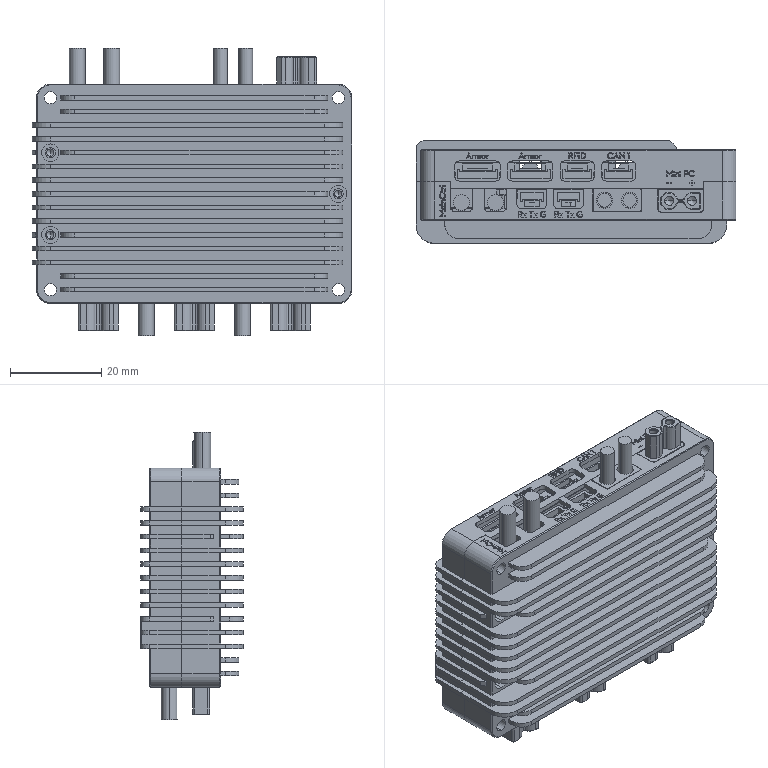Part | SolidWorks | features BaseBody 46, ICE 1 | 37 solids | 7107 faces | volume 27564 mm3 | plane 4212 | spline 1700 | cylinder 1072 | cone 123 | commonest cylinder face diameters 1 x131 2.5 x123 2 x100 3.5 x94 1.4 x64 0.9 x48